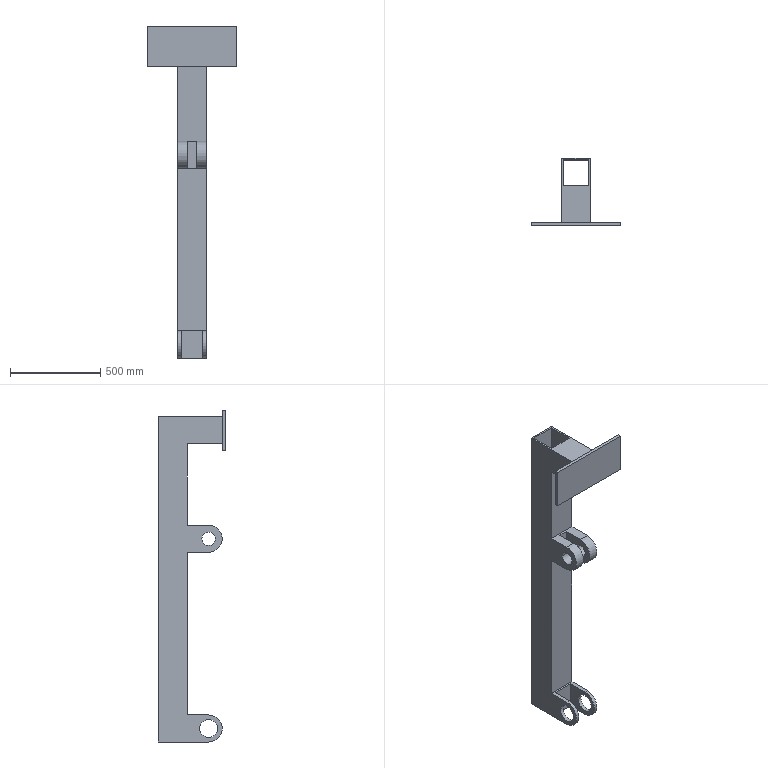Part | SolidWorks | features BaseBody 1 | 1 solid | 39 faces | box 495 x 375.221 x 1838 mm | volume 21198694 mm3 | plane 27 | cylinder 12 | commonest cylinder face diameters 75 x4 100 x4 150 x4
STEP:
#1=CARTESIAN_POINT('',(25.,-237.5,1125.));
#2=VERTEX_POINT('',#1);
#3=CARTESIAN_POINT('',(25.,-162.5,1125.));
#4=VERTEX_POINT('',#3);
#5=CARTESIAN_POINT('',(25.,-200.,1125.));
#6=DIRECTION('',(1.,0.,0.));
#7=DIRECTION('',(0.,1.,0.));
#8=AXIS2_PLACEMENT_3D('',#5,#6,#7);
#9=CIRCLE('',#8,37.5);
#10=EDGE_CURVE('',#2,#4,#9,.T.);
#11=ORIENTED_EDGE('',*,*,#10,.F.);
#12=CARTESIAN_POINT('',(80.,-237.5,1125.));
#13=VERTEX_POINT('',#12);
#14=CARTESIAN_POINT('',(-289.,-237.5,1125.));
#15=DIRECTION('',(1.,0.,0.));
#16=VECTOR('',#15,1000.);
#17=LINE('',#14,#16);
#18=EDGE_CURVE('',#2,#13,#17,.T.);
#19=ORIENTED_EDGE('',*,*,#18,.T.);
#20=CARTESIAN_POINT('',(80.,-162.5,1125.));
#21=VERTEX_POINT('',#20);
#22=CARTESIAN_POINT('',(80.,-200.,1125.));
#23=DIRECTION('',(1.,0.,0.));
#24=DIRECTION('',(0.,1.,0.));
#25=AXIS2_PLACEMENT_3D('',#22,#23,#24);
#26=CIRCLE('',#25,37.5);
#27=EDGE_CURVE('',#13,#21,#26,.T.);
#28=ORIENTED_EDGE('',*,*,#27,.T.);
#29=CARTESIAN_POINT('',(-289.,-162.5,1125.));
#30=DIRECTION('',(1.,0.,0.));
#31=VECTOR('',#30,1000.);
#32=LINE('',#29,#31);
#33=EDGE_CURVE('',#4,#21,#32,.T.);
#34=ORIENTED_EDGE('',*,*,#33,.F.);
#35=EDGE_LOOP('',(#11,#19,#28,#34));
#36=FACE_OUTER_BOUND('',#35,.T.);
#37=CARTESIAN_POINT('',(-289.,-200.,1125.));
#38=DIRECTION('',(1.,0.,0.));
#39=DIRECTION('',(0.,1.,0.));
#40=AXIS2_PLACEMENT_3D('',#37,#38,#39);
#41=CYLINDRICAL_SURFACE('',#40,37.5);
#42=ADVANCED_FACE('',(#36),#41,.F.);
#43=CARTESIAN_POINT('',(60.,-250.,75.));
#44=VERTEX_POINT('',#43);
#45=CARTESIAN_POINT('',(60.,-150.,75.));
#46=VERTEX_POINT('',#45);
#47=CARTESIAN_POINT('',(60.,-200.,75.));
#48=DIRECTION('',(1.,0.,0.));
#49=DIRECTION('',(0.,1.,0.));
#50=AXIS2_PLACEMENT_3D('',#47,#48,#49);
#51=CIRCLE('',#50,50.);
#52=EDGE_CURVE('',#44,#46,#51,.T.);
#53=ORIENTED_EDGE('',*,*,#52,.F.);
#54=CARTESIAN_POINT('',(80.,-250.,75.));
#55=VERTEX_POINT('',#54);
#56=CARTESIAN_POINT('',(-2456.,-250.,75.));
#57=DIRECTION('',(1.,0.,0.));
#58=VECTOR('',#57,1000.);
#59=LINE('',#56,#58);
#60=EDGE_CURVE('',#44,#55,#59,.T.);
#61=ORIENTED_EDGE('',*,*,#60,.T.);
#62=CARTESIAN_POINT('',(80.,-150.,75.));
#63=VERTEX_POINT('',#62);
#64=CARTESIAN_POINT('',(80.,-200.,75.));
#65=DIRECTION('',(1.,0.,0.));
#66=DIRECTION('',(0.,1.,0.));
#67=AXIS2_PLACEMENT_3D('',#64,#65,#66);
#68=CIRCLE('',#67,50.);
#69=EDGE_CURVE('',#55,#63,#68,.T.);
#70=ORIENTED_EDGE('',*,*,#69,.T.);
#71=CARTESIAN_POINT('',(-2456.,-150.,75.));
#72=DIRECTION('',(1.,0.,0.));
#73=VECTOR('',#72,1000.);
#74=LINE('',#71,#73);
#75=EDGE_CURVE('',#46,#63,#74,.T.);
#76=ORIENTED_EDGE('',*,*,#75,.F.);
#77=EDGE_LOOP('',(#53,#61,#70,#76));
#78=FACE_OUTER_BOUND('',#77,.T.);
#79=CARTESIAN_POINT('',(-2456.,-200.,75.));
#80=DIRECTION('',(1.,0.,0.));
#81=DIRECTION('',(0.,1.,0.));
#82=AXIS2_PLACEMENT_3D('',#79,#80,#81);
#83=CYLINDRICAL_SURFACE('',#82,50.);
#84=ADVANCED_FACE('',(#78),#83,.F.);
#85=CARTESIAN_POINT('',(-80.,-162.5,1125.));
#86=VERTEX_POINT('',#85);
#87=CARTESIAN_POINT('',(-80.,-237.5,1125.));
#88=VERTEX_POINT('',#87);
#89=CARTESIAN_POINT('',(-80.,-200.,1125.));
#90=DIRECTION('',(-1.,0.,0.));
#91=DIRECTION('',(0.,1.,0.));
#92=AXIS2_PLACEMENT_3D('',#89,#90,#91);
#93=CIRCLE('',#92,37.5);
#94=EDGE_CURVE('',#86,#88,#93,.T.);
#95=ORIENTED_EDGE('',*,*,#94,.T.);
#96=CARTESIAN_POINT('',(-25.,-237.5,1125.));
#97=VERTEX_POINT('',#96);
#98=CARTESIAN_POINT('',(-289.,-237.5,1125.));
#99=DIRECTION('',(1.,0.,0.));
#100=VECTOR('',#99,1000.);
#101=LINE('',#98,#100);
#102=EDGE_CURVE('',#88,#97,#101,.T.);
#103=ORIENTED_EDGE('',*,*,#102,.T.);
#104=CARTESIAN_POINT('',(-25.,-162.5,1125.));
#105=VERTEX_POINT('',#104);
#106=CARTESIAN_POINT('',(-25.,-200.,1125.));
#107=DIRECTION('',(-1.,0.,0.));
#108=DIRECTION('',(0.,1.,0.));
#109=AXIS2_PLACEMENT_3D('',#106,#107,#108);
#110=CIRCLE('',#109,37.5);
#111=EDGE_CURVE('',#105,#97,#110,.T.);
#112=ORIENTED_EDGE('',*,*,#111,.F.);
#113=CARTESIAN_POINT('',(-289.,-162.5,1125.));
#114=DIRECTION('',(1.,0.,0.));
#115=VECTOR('',#114,1000.);
#116=LINE('',#113,#115);
#117=EDGE_CURVE('',#86,#105,#116,.T.);
#118=ORIENTED_EDGE('',*,*,#117,.F.);
#119=EDGE_LOOP('',(#95,#103,#112,#118));
#120=FACE_OUTER_BOUND('',#119,.T.);
#121=CARTESIAN_POINT('',(-289.,-200.,1125.));
#122=DIRECTION('',(1.,0.,0.));
#123=DIRECTION('',(0.,1.,0.));
#124=AXIS2_PLACEMENT_3D('',#121,#122,#123);
#125=CYLINDRICAL_SURFACE('',#124,37.5);
#126=ADVANCED_FACE('',(#120),#125,.F.);
#127=CARTESIAN_POINT('',(-80.,-150.,75.));
#128=VERTEX_POINT('',#127);
#129=CARTESIAN_POINT('',(-80.,-250.,75.));
#130=VERTEX_POINT('',#129);
#131=CARTESIAN_POINT('',(-80.,-200.,75.));
#132=DIRECTION('',(-1.,0.,0.));
#133=DIRECTION('',(0.,1.,0.));
#134=AXIS2_PLACEMENT_3D('',#131,#132,#133);
#135=CIRCLE('',#134,50.);
#136=EDGE_CURVE('',#128,#130,#135,.T.);
#137=ORIENTED_EDGE('',*,*,#136,.T.);
#138=CARTESIAN_POINT('',(-60.,-250.,75.));
#139=VERTEX_POINT('',#138);
#140=CARTESIAN_POINT('',(-2456.,-250.,75.));
#141=DIRECTION('',(1.,0.,0.));
#142=VECTOR('',#141,1000.);
#143=LINE('',#140,#142);
#144=EDGE_CURVE('',#130,#139,#143,.T.);
#145=ORIENTED_EDGE('',*,*,#144,.T.);
#146=CARTESIAN_POINT('',(-60.,-150.,75.));
#147=VERTEX_POINT('',#146);
#148=CARTESIAN_POINT('',(-60.,-200.,75.));
#149=DIRECTION('',(1.,0.,0.));
#150=DIRECTION('',(0.,1.,0.));
#151=AXIS2_PLACEMENT_3D('',#148,#149,#150);
#152=CIRCLE('',#151,50.);
#153=EDGE_CURVE('',#139,#147,#152,.T.);
#154=ORIENTED_EDGE('',*,*,#153,.T.);
#155=CARTESIAN_POINT('',(-2456.,-150.,75.));
#156=DIRECTION('',(1.,0.,0.));
#157=VECTOR('',#156,1000.);
#158=LINE('',#155,#157);
#159=EDGE_CURVE('',#128,#147,#158,.T.);
#160=ORIENTED_EDGE('',*,*,#159,.F.);
#161=EDGE_LOOP('',(#137,#145,#154,#160));
#162=FACE_OUTER_BOUND('',#161,.T.);
#163=CARTESIAN_POINT('',(-2456.,-200.,75.));
#164=DIRECTION('',(1.,0.,0.));
#165=DIRECTION('',(0.,1.,0.));
#166=AXIS2_PLACEMENT_3D('',#163,#164,#165);
#167=CYLINDRICAL_SURFACE('',#166,50.);
#168=ADVANCED_FACE('',(#162),#167,.F.);
#169=CARTESIAN_POINT('',(80.,-200.,1125.));
#170=DIRECTION('',(1.,0.,0.));
#171=DIRECTION('',(0.,1.,0.));
#172=AXIS2_PLACEMENT_3D('',#169,#170,#171);
#173=CIRCLE('',#172,37.5);
#174=EDGE_CURVE('',#21,#13,#173,.T.);
#175=ORIENTED_EDGE('',*,*,#174,.F.);
#176=ORIENTED_EDGE('',*,*,#27,.F.);
#177=EDGE_LOOP('',(#175,#176));
#178=FACE_BOUND('',#177,.T.);
#179=CARTESIAN_POINT('',(80.,-200.,75.));
#180=DIRECTION('',(1.,0.,0.));
#181=DIRECTION('',(0.,1.,0.));
#182=AXIS2_PLACEMENT_3D('',#179,#180,#181);
#183=CIRCLE('',#182,50.);
#184=EDGE_CURVE('',#63,#55,#183,.T.);
#185=ORIENTED_EDGE('',*,*,#184,.F.);
#186=ORIENTED_EDGE('',*,*,#69,.F.);
#187=EDGE_LOOP('',(#185,#186));
#188=FACE_BOUND('',#187,.T.);
#189=CARTESIAN_POINT('',(80.,-80.,1200.));
#190=VERTEX_POINT('',#189);
#191=CARTESIAN_POINT('',(80.,-80.,1650.));
#192=VERTEX_POINT('',#191);
#193=CARTESIAN_POINT('',(80.,-80.,1800.));
#194=DIRECTION('',(0.,0.,1.));
#195=VECTOR('',#194,1000.);
#196=LINE('',#193,#195);
#197=EDGE_CURVE('',#190,#192,#196,.T.);
#198=ORIENTED_EDGE('',*,*,#197,.F.);
#199=CARTESIAN_POINT('',(80.,-200.,1200.));
#200=VERTEX_POINT('',#199);
#201=CARTESIAN_POINT('',(80.,-80.,1200.));
#202=DIRECTION('',(0.,1.,0.));
#203=VECTOR('',#202,1000.);
#204=LINE('',#201,#203);
#205=EDGE_CURVE('',#200,#190,#204,.T.);
#206=ORIENTED_EDGE('',*,*,#205,.F.);
#207=CARTESIAN_POINT('',(80.,-200.,1050.));
#208=VERTEX_POINT('',#207);
#209=CARTESIAN_POINT('',(80.,-200.,1125.));
#210=DIRECTION('',(-1.,0.,0.));
#211=DIRECTION('',(0.,1.,0.));
#212=AXIS2_PLACEMENT_3D('',#209,#210,#211);
#213=CIRCLE('',#212,75.);
#214=EDGE_CURVE('',#208,#200,#213,.T.);
#215=ORIENTED_EDGE('',*,*,#214,.F.);
#216=CARTESIAN_POINT('',(80.,-80.,1050.));
#217=VERTEX_POINT('',#216);
#218=CARTESIAN_POINT('',(80.,-80.,1050.));
#219=DIRECTION('',(0.,-1.,0.));
#220=VECTOR('',#219,1000.);
#221=LINE('',#218,#220);
#222=EDGE_CURVE('',#217,#208,#221,.T.);
#223=ORIENTED_EDGE('',*,*,#222,.F.);
#224=CARTESIAN_POINT('',(80.,-80.,150.));
#225=VERTEX_POINT('',#224);
#226=CARTESIAN_POINT('',(80.,-80.,1800.));
#227=DIRECTION('',(0.,0.,1.));
#228=VECTOR('',#227,1000.);
#229=LINE('',#226,#228);
#230=EDGE_CURVE('',#225,#217,#229,.T.);
#231=ORIENTED_EDGE('',*,*,#230,.F.);
#232=CARTESIAN_POINT('',(80.,-200.,150.));
#233=VERTEX_POINT('',#232);
#234=CARTESIAN_POINT('',(80.,-80.,150.));
#235=DIRECTION('',(0.,1.,0.));
#236=VECTOR('',#235,1000.);
#237=LINE('',#234,#236);
#238=EDGE_CURVE('',#233,#225,#237,.T.);
#239=ORIENTED_EDGE('',*,*,#238,.F.);
#240=CARTESIAN_POINT('',(80.,-200.,0.));
#241=VERTEX_POINT('',#240);
#242=CARTESIAN_POINT('',(80.,-200.,75.));
#243=DIRECTION('',(-1.,0.,0.));
#244=DIRECTION('',(0.,1.,0.));
#245=AXIS2_PLACEMENT_3D('',#242,#243,#244);
#246=CIRCLE('',#245,75.);
#247=EDGE_CURVE('',#241,#233,#246,.T.);
#248=ORIENTED_EDGE('',*,*,#247,.F.);
#249=CARTESIAN_POINT('',(80.,80.,0.));
#250=VERTEX_POINT('',#249);
#251=CARTESIAN_POINT('',(80.,-80.,0.));
#252=DIRECTION('',(0.,-1.,0.));
#253=VECTOR('',#252,1000.);
#254=LINE('',#251,#253);
#255=EDGE_CURVE('',#250,#241,#254,.T.);
#256=ORIENTED_EDGE('',*,*,#255,.F.);
#257=CARTESIAN_POINT('',(80.,80.,1800.));
#258=VERTEX_POINT('',#257);
#259=CARTESIAN_POINT('',(80.,80.,1800.));
#260=DIRECTION('',(0.,0.,-1.));
#261=VECTOR('',#260,1000.);
#262=LINE('',#259,#261);
#263=EDGE_CURVE('',#258,#250,#262,.T.);
#264=ORIENTED_EDGE('',*,*,#263,.F.);
#265=CARTESIAN_POINT('',(80.,-275.221,1800.));
#266=VERTEX_POINT('',#265);
#267=CARTESIAN_POINT('',(80.,-80.,1800.));
#268=DIRECTION('',(0.,1.,0.));
#269=VECTOR('',#268,1000.);
#270=LINE('',#267,#269);
#271=EDGE_CURVE('',#266,#258,#270,.T.);
#272=ORIENTED_EDGE('',*,*,#271,.F.);
#273=CARTESIAN_POINT('',(80.,-275.221,1650.));
#274=VERTEX_POINT('',#273);
#275=CARTESIAN_POINT('',(80.,-275.221,1800.));
#276=DIRECTION('',(0.,0.,1.));
#277=VECTOR('',#276,1000.);
#278=LINE('',#275,#277);
#279=EDGE_CURVE('',#274,#266,#278,.T.);
#280=ORIENTED_EDGE('',*,*,#279,.F.);
#281=CARTESIAN_POINT('',(80.,-80.,1650.));
#282=DIRECTION('',(0.,-1.,0.));
#283=VECTOR('',#282,1000.);
#284=LINE('',#281,#283);
#285=EDGE_CURVE('',#192,#274,#284,.T.);
#286=ORIENTED_EDGE('',*,*,#285,.F.);
#287=EDGE_LOOP('',(#198,#206,#215,#223,#231,#239,#248,#256,#264,#272,#280,#286));
#288=FACE_OUTER_BOUND('',#287,.T.);
#289=CARTESIAN_POINT('',(80.,-80.,1800.));
#290=DIRECTION('',(-1.,0.,0.));
#291=DIRECTION('',(0.,-1.,0.));
#292=AXIS2_PLACEMENT_3D('',#289,#290,#291);
#293=PLANE('',#292);
#294=ADVANCED_FACE('',(#178,#188,#288),#293,.F.);
#295=ORIENTED_EDGE('',*,*,#18,.F.);
#296=CARTESIAN_POINT('',(25.,-200.,1125.));
#297=DIRECTION('',(1.,0.,0.));
#298=DIRECTION('',(0.,1.,0.));
#299=AXIS2_PLACEMENT_3D('',#296,#297,#298);
#300=CIRCLE('',#299,37.5);
#301=EDGE_CURVE('',#4,#2,#300,.T.);
#302=ORIENTED_EDGE('',*,*,#301,.F.);
#303=ORIENTED_EDGE('',*,*,#33,.T.);
#304=ORIENTED_EDGE('',*,*,#174,.T.);
#305=EDGE_LOOP('',(#295,#302,#303,#304));
#306=FACE_OUTER_BOUND('',#305,.T.);
#307=CARTESIAN_POINT('',(-289.,-200.,1125.));
#308=DIRECTION('',(1.,0.,0.));
#309=DIRECTION('',(0.,1.,0.));
#310=AXIS2_PLACEMENT_3D('',#307,#308,#309);
#311=CYLINDRICAL_SURFACE('',#310,37.5);
#312=ADVANCED_FACE('',(#306),#311,.F.);
#313=ORIENTED_EDGE('',*,*,#60,.F.);
#314=CARTESIAN_POINT('',(60.,-200.,75.));
#315=DIRECTION('',(1.,0.,0.));
#316=DIRECTION('',(0.,1.,0.));
#317=AXIS2_PLACEMENT_3D('',#314,#315,#316);
#318=CIRCLE('',#317,50.);
#319=EDGE_CURVE('',#46,#44,#318,.T.);
#320=ORIENTED_EDGE('',*,*,#319,.F.);
#321=ORIENTED_EDGE('',*,*,#75,.T.);
#322=ORIENTED_EDGE('',*,*,#184,.T.);
#323=EDGE_LOOP('',(#313,#320,#321,#322));
#324=FACE_OUTER_BOUND('',#323,.T.);
#325=CARTESIAN_POINT('',(-2456.,-200.,75.));
#326=DIRECTION('',(1.,0.,0.));
#327=DIRECTION('',(0.,1.,0.));
#328=AXIS2_PLACEMENT_3D('',#325,#326,#327);
#329=CYLINDRICAL_SURFACE('',#328,50.);
#330=ADVANCED_FACE('',(#324),#329,.F.);
#331=ORIENTED_EDGE('',*,*,#285,.T.);
#332=CARTESIAN_POINT('',(-80.,-275.221,1650.));
#333=VERTEX_POINT('',#332);
#334=CARTESIAN_POINT('',(-80.,-275.221,1650.));
#335=DIRECTION('',(-1.,0.,0.));
#336=VECTOR('',#335,1000.);
#337=LINE('',#334,#336);
#338=EDGE_CURVE('',#274,#333,#337,.T.);
#339=ORIENTED_EDGE('',*,*,#338,.T.);
#340=CARTESIAN_POINT('',(-80.,-80.,1650.));
#341=VERTEX_POINT('',#340);
#342=CARTESIAN_POINT('',(-80.,-200.,1650.));
#343=DIRECTION('',(0.,1.,0.));
#344=VECTOR('',#343,1000.);
#345=LINE('',#342,#344);
#346=EDGE_CURVE('',#333,#341,#345,.T.);
#347=ORIENTED_EDGE('',*,*,#346,.T.);
#348=CARTESIAN_POINT('',(-80.,-80.,1650.));
#349=DIRECTION('',(1.,0.,0.));
#350=VECTOR('',#349,1000.);
#351=LINE('',#348,#350);
#352=EDGE_CURVE('',#341,#192,#351,.T.);
#353=ORIENTED_EDGE('',*,*,#352,.T.);
#354=EDGE_LOOP('',(#331,#339,#347,#353));
#355=FACE_OUTER_BOUND('',#354,.T.);
#356=CARTESIAN_POINT('',(-80.,-200.,1650.));
#357=DIRECTION('',(0.,0.,-1.));
#358=DIRECTION('',(0.,1.,0.));
#359=AXIS2_PLACEMENT_3D('',#356,#357,#358);
#360=PLANE('',#359);
#361=ADVANCED_FACE('',(#355),#360,.T.);
#362=ORIENTED_EDGE('',*,*,#352,.F.);
#363=CARTESIAN_POINT('',(-80.,-80.,1200.));
#364=VERTEX_POINT('',#363);
#365=CARTESIAN_POINT('',(-80.,-80.,1800.));
#366=DIRECTION('',(0.,0.,1.));
#367=VECTOR('',#366,1000.);
#368=LINE('',#365,#367);
#369=EDGE_CURVE('',#364,#341,#368,.T.);
#370=ORIENTED_EDGE('',*,*,#369,.F.);
#371=CARTESIAN_POINT('',(80.,-80.,1200.));
#372=DIRECTION('',(-1.,0.,0.));
#373=VECTOR('',#372,1000.);
#374=LINE('',#371,#373);
#375=EDGE_CURVE('',#190,#364,#374,.T.);
#376=ORIENTED_EDGE('',*,*,#375,.F.);
#377=ORIENTED_EDGE('',*,*,#197,.T.);
#378=EDGE_LOOP('',(#362,#370,#376,#377));
#379=FACE_OUTER_BOUND('',#378,.T.);
#380=CARTESIAN_POINT('',(80.,-80.,1800.));
#381=DIRECTION('',(0.,1.,0.));
#382=DIRECTION('',(-1.,0.,0.));
#383=AXIS2_PLACEMENT_3D('',#380,#381,#382);
#384=PLANE('',#383);
#385=ADVANCED_FACE('',(#379),#384,.F.);
#386=CARTESIAN_POINT('',(-80.,-200.,1200.));
#387=VERTEX_POINT('',#386);
#388=CARTESIAN_POINT('',(-25.,-200.,1200.));
#389=VERTEX_POINT('',#388);
#390=CARTESIAN_POINT('',(-80.,-200.,1200.));
#391=DIRECTION('',(1.,0.,0.));
#392=VECTOR('',#391,1000.);
#393=LINE('',#390,#392);
#394=EDGE_CURVE('',#387,#389,#393,.T.);
#395=ORIENTED_EDGE('',*,*,#394,.T.);
#396=CARTESIAN_POINT('',(-25.,-90.221,1200.));
#397=VERTEX_POINT('',#396);
#398=CARTESIAN_POINT('',(-25.,-80.,1200.));
#399=DIRECTION('',(0.,1.,0.));
#400=VECTOR('',#399,1000.);
#401=LINE('',#398,#400);
#402=EDGE_CURVE('',#389,#397,#401,.T.);
#403=ORIENTED_EDGE('',*,*,#402,.T.);
#404=CARTESIAN_POINT('',(25.,-90.221,1200.));
#405=VERTEX_POINT('',#404);
#406=CARTESIAN_POINT('',(-80.,-90.221,1200.));
#407=DIRECTION('',(1.,0.,0.));
#408=VECTOR('',#407,1000.);
#409=LINE('',#406,#408);
#410=EDGE_CURVE('',#397,#405,#409,.T.);
#411=ORIENTED_EDGE('',*,*,#410,.T.);
#412=CARTESIAN_POINT('',(25.,-200.,1200.));
#413=VERTEX_POINT('',#412);
#414=CARTESIAN_POINT('',(25.,-80.,1200.));
#415=DIRECTION('',(0.,-1.,0.));
#416=VECTOR('',#415,1000.);
#417=LINE('',#414,#416);
#418=EDGE_CURVE('',#405,#413,#417,.T.);
#419=ORIENTED_EDGE('',*,*,#418,.T.);
#420=CARTESIAN_POINT('',(-80.,-200.,1200.));
#421=DIRECTION('',(1.,0.,0.));
#422=VECTOR('',#421,1000.);
#423=LINE('',#420,#422);
#424=EDGE_CURVE('',#413,#200,#423,.T.);
#425=ORIENTED_EDGE('',*,*,#424,.T.);
#426=ORIENTED_EDGE('',*,*,#205,.T.);
#427=ORIENTED_EDGE('',*,*,#375,.T.);
#428=CARTESIAN_POINT('',(-80.,-80.,1200.));
#429=DIRECTION('',(0.,-1.,0.));
#430=VECTOR('',#429,1000.);
#431=LINE('',#428,#430);
#432=EDGE_CURVE('',#364,#387,#431,.T.);
#433=ORIENTED_EDGE('',*,*,#432,.T.);
#434=EDGE_LOOP('',(#395,#403,#411,#419,#425,#426,#427,#433));
#435=FACE_OUTER_BOUND('',#434,.T.);
#436=CARTESIAN_POINT('',(-80.,-80.,1200.));
#437=DIRECTION('',(0.,0.,1.));
#438=DIRECTION('',(0.,-1.,0.));
#439=AXIS2_PLACEMENT_3D('',#436,#437,#438);
#440=PLANE('',#439);
#441=ADVANCED_FACE('',(#435),#440,.T.);
#442=CARTESIAN_POINT('',(25.,-200.,1050.));
#443=VERTEX_POINT('',#442);
#444=CARTESIAN_POINT('',(-80.,-200.,1050.));
#445=DIRECTION('',(1.,0.,0.));
#446=VECTOR('',#445,1000.);
#447=LINE('',#444,#446);
#448=EDGE_CURVE('',#443,#208,#447,.T.);
#449=ORIENTED_EDGE('',*,*,#448,.T.);
#450=ORIENTED_EDGE('',*,*,#214,.T.);
#451=ORIENTED_EDGE('',*,*,#424,.F.);
#452=CARTESIAN_POINT('',(25.,-200.,1125.));
#453=DIRECTION('',(1.,0.,0.));
#454=DIRECTION('',(0.,1.,0.));
#455=AXIS2_PLACEMENT_3D('',#452,#453,#454);
#456=CIRCLE('',#455,75.);
#457=EDGE_CURVE('',#413,#443,#456,.T.);
#458=ORIENTED_EDGE('',*,*,#457,.T.);
#459=EDGE_LOOP('',(#449,#450,#451,#458));
#460=FACE_OUTER_BOUND('',#459,.T.);
#461=CARTESIAN_POINT('',(-80.,-200.,1125.));
#462=DIRECTION('',(1.,0.,0.));
#463=DIRECTION('',(0.,1.,0.));
#464=AXIS2_PLACEMENT_3D('',#461,#462,#463);
#465=CYLINDRICAL_SURFACE('',#464,75.);
#466=ADVANCED_FACE('',(#460),#465,.T.);
#467=CARTESIAN_POINT('',(-80.,-80.,1050.));
#468=VERTEX_POINT('',#467);
#469=CARTESIAN_POINT('',(-80.,-80.,1050.));
#470=DIRECTION('',(1.,0.,0.));
#471=VECTOR('',#470,1000.);
#472=LINE('',#469,#471);
#473=EDGE_CURVE('',#468,#217,#472,.T.);
#474=ORIENTED_EDGE('',*,*,#473,.T.);
#475=ORIENTED_EDGE('',*,*,#222,.T.);
#476=ORIENTED_EDGE('',*,*,#448,.F.);
#477=CARTESIAN_POINT('',(25.,-90.221,1050.));
#478=VERTEX_POINT('',#477);
#479=CARTESIAN_POINT('',(25.,-200.,1050.));
#480=DIRECTION('',(0.,1.,0.));
#481=VECTOR('',#480,1000.);
#482=LINE('',#479,#481);
#483=EDGE_CURVE('',#443,#478,#482,.T.);
#484=ORIENTED_EDGE('',*,*,#483,.T.);
#485=CARTESIAN_POINT('',(-25.,-90.221,1050.));
#486=VERTEX_POINT('',#485);
#487=CARTESIAN_POINT('',(-80.,-90.221,1050.));
#488=DIRECTION('',(-1.,0.,0.));
#489=VECTOR('',#488,1000.);
#490=LINE('',#487,#489);
#491=EDGE_CURVE('',#478,#486,#490,.T.);
#492=ORIENTED_EDGE('',*,*,#491,.T.);
#493=CARTESIAN_POINT('',(-25.,-200.,1050.));
#494=VERTEX_POINT('',#493);
#495=CARTESIAN_POINT('',(-25.,-200.,1050.));
#496=DIRECTION('',(0.,-1.,0.));
#497=VECTOR('',#496,1000.);
#498=LINE('',#495,#497);
#499=EDGE_CURVE('',#486,#494,#498,.T.);
#500=ORIENTED_EDGE('',*,*,#499,.T.);
#501=CARTESIAN_POINT('',(-80.,-200.,1050.));
#502=VERTEX_POINT('',#501);
#503=CARTESIAN_POINT('',(-80.,-200.,1050.));
#504=DIRECTION('',(-1.,0.,0.));
#505=VECTOR('',#504,1000.);
#506=LINE('',#503,#505);
#507=EDGE_CURVE('',#494,#502,#506,.T.);
#508=ORIENTED_EDGE('',*,*,#507,.T.);
#509=CARTESIAN_POINT('',(-80.,-200.,1050.));
#510=DIRECTION('',(0.,1.,0.));
#511=VECTOR('',#510,1000.);
#512=LINE('',#509,#511);
#513=EDGE_CURVE('',#502,#468,#512,.T.);
#514=ORIENTED_EDGE('',*,*,#513,.T.);
#515=EDGE_LOOP('',(#474,#475,#476,#484,#492,#500,#508,#514));
#516=FACE_OUTER_BOUND('',#515,.T.);
#517=CARTESIAN_POINT('',(-80.,-200.,1050.));
#518=DIRECTION('',(0.,0.,-1.));
#519=DIRECTION('',(-1.,0.,0.));
#520=AXIS2_PLACEMENT_3D('',#517,#518,#519);
#521=PLANE('',#520);
#522=ADVANCED_FACE('',(#516),#521,.T.);
#523=ORIENTED_EDGE('',*,*,#473,.F.);
#524=CARTESIAN_POINT('',(-80.,-80.,150.));
#525=VERTEX_POINT('',#524);
#526=CARTESIAN_POINT('',(-80.,-80.,1800.));
#527=DIRECTION('',(0.,0.,1.));
#528=VECTOR('',#527,1000.);
#529=LINE('',#526,#528);
#530=EDGE_CURVE('',#525,#468,#529,.T.);
#531=ORIENTED_EDGE('',*,*,#530,.F.);
#532=CARTESIAN_POINT('',(80.,-80.,150.));
#533=DIRECTION('',(-1.,0.,0.));
#534=VECTOR('',#533,1000.);
#535=LINE('',#532,#534);
#536=EDGE_CURVE('',#225,#525,#535,.T.);
#537=ORIENTED_EDGE('',*,*,#536,.F.);
#538=ORIENTED_EDGE('',*,*,#230,.T.);
#539=EDGE_LOOP('',(#523,#531,#537,#538));
#540=FACE_OUTER_BOUND('',#539,.T.);
#541=CARTESIAN_POINT('',(80.,-80.,1800.));
#542=DIRECTION('',(0.,1.,0.));
#543=DIRECTION('',(-1.,0.,0.));
#544=AXIS2_PLACEMENT_3D('',#541,#542,#543);
#545=PLANE('',#544);
#546=ADVANCED_FACE('',(#540),#545,.F.);
#547=CARTESIAN_POINT('',(-60.,-200.,150.));
#548=VERTEX_POINT('',#547);
#549=CARTESIAN_POINT('',(-60.,-90.221,150.));
#550=VERTEX_POINT('',#549);
#551=CARTESIAN_POINT('',(-60.,-200.,150.));
#552=DIRECTION('',(0.,1.,0.));
#553=VECTOR('',#552,1000.);
#554=LINE('',#551,#553);
#555=EDGE_CURVE('',#548,#550,#554,.T.);
#556=ORIENTED_EDGE('',*,*,#555,.T.);
#557=CARTESIAN_POINT('',(60.,-90.221,150.));
#558=VERTEX_POINT('',#557);
#559=CARTESIAN_POINT('',(-80.,-90.221,150.));
#560=DIRECTION('',(1.,0.,0.));
#561=VECTOR('',#560,1000.);
#562=LINE('',#559,#561);
#563=EDGE_CURVE('',#550,#558,#562,.T.);
#564=ORIENTED_EDGE('',*,*,#563,.T.);
#565=CARTESIAN_POINT('',(60.,-200.,150.));
#566=VERTEX_POINT('',#565);
#567=CARTESIAN_POINT('',(60.,-200.,150.));
#568=DIRECTION('',(0.,-1.,0.));
#569=VECTOR('',#568,1000.);
#570=LINE('',#567,#569);
#571=EDGE_CURVE('',#558,#566,#570,.T.);
#572=ORIENTED_EDGE('',*,*,#571,.T.);
#573=CARTESIAN_POINT('',(-80.,-200.,150.));
#574=DIRECTION('',(1.,0.,0.));
#575=VECTOR('',#574,1000.);
#576=LINE('',#573,#575);
#577=EDGE_CURVE('',#566,#233,#576,.T.);
#578=ORIENTED_EDGE('',*,*,#577,.T.);
#579=ORIENTED_EDGE('',*,*,#238,.T.);
#580=ORIENTED_EDGE('',*,*,#536,.T.);
#581=CARTESIAN_POINT('',(-80.,-200.,150.));
#582=VERTEX_POINT('',#581);
#583=CARTESIAN_POINT('',(-80.,-200.,150.));
#584=DIRECTION('',(0.,-1.,0.));
#585=VECTOR('',#584,1000.);
#586=LINE('',#583,#585);
#587=EDGE_CURVE('',#525,#582,#586,.T.);
#588=ORIENTED_EDGE('',*,*,#587,.T.);
#589=CARTESIAN_POINT('',(-80.,-200.,150.));
#590=DIRECTION('',(1.,0.,0.));
#591=VECTOR('',#590,1000.);
#592=LINE('',#589,#591);
#593=EDGE_CURVE('',#582,#548,#592,.T.);
#594=ORIENTED_EDGE('',*,*,#593,.T.);
#595=EDGE_LOOP('',(#556,#564,#572,#578,#579,#580,#588,#594));
#596=FACE_OUTER_BOUND('',#595,.T.);
#597=CARTESIAN_POINT('',(-80.,-200.,150.));
#598=DIRECTION('',(0.,0.,1.));
#599=DIRECTION('',(0.,-1.,0.));
#600=AXIS2_PLACEMENT_3D('',#597,#598,#599);
#601=PLANE('',#600);
#602=ADVANCED_FACE('',(#596),#601,.T.);
#603=ORIENTED_EDGE('',*,*,#247,.T.);
#604=ORIENTED_EDGE('',*,*,#577,.F.);
#605=CARTESIAN_POINT('',(60.,-200.,0.));
#606=VERTEX_POINT('',#605);
#607=CARTESIAN_POINT('',(60.,-200.,75.));
#608=DIRECTION('',(1.,0.,0.));
#609=DIRECTION('',(0.,1.,0.));
#610=AXIS2_PLACEMENT_3D('',#607,#608,#609);
#611=CIRCLE('',#610,75.);
#612=EDGE_CURVE('',#566,#606,#611,.T.);
#613=ORIENTED_EDGE('',*,*,#612,.T.);
#614=CARTESIAN_POINT('',(-80.,-200.,0.));
#615=DIRECTION('',(1.,0.,0.));
#616=VECTOR('',#615,1000.);
#617=LINE('',#614,#616);
#618=EDGE_CURVE('',#606,#241,#617,.T.);
#619=ORIENTED_EDGE('',*,*,#618,.T.);
#620=EDGE_LOOP('',(#603,#604,#613,#619));
#621=FACE_OUTER_BOUND('',#620,.T.);
#622=CARTESIAN_POINT('',(-80.,-200.,75.));
#623=DIRECTION('',(1.,0.,0.));
#624=DIRECTION('',(0.,1.,0.));
#625=AXIS2_PLACEMENT_3D('',#622,#623,#624);
#626=CYLINDRICAL_SURFACE('',#625,75.);
#627=ADVANCED_FACE('',(#621),#626,.T.);
#628=CARTESIAN_POINT('',(-70.,70.,0.));
#629=VERTEX_POINT('',#628);
#630=CARTESIAN_POINT('',(70.,70.,0.));
#631=VERTEX_POINT('',#630);
#632=CARTESIAN_POINT('',(0.,70.,0.));
#633=DIRECTION('',(1.,0.,0.));
#634=VECTOR('',#633,1000.);
#635=LINE('',#632,#634);
#636=EDGE_CURVE('',#629,#631,#635,.T.);
#637=ORIENTED_EDGE('',*,*,#636,.F.);
#638=CARTESIAN_POINT('',(-70.,-70.,0.));
#639=VERTEX_POINT('',#638);
#640=CARTESIAN_POINT('',(-70.,0.,0.));
#641=DIRECTION('',(0.,1.,0.));
#642=VECTOR('',#641,1000.);
#643=LINE('',#640,#642);
#644=EDGE_CURVE('',#639,#629,#643,.T.);
#645=ORIENTED_EDGE('',*,*,#644,.F.);
#646=CARTESIAN_POINT('',(70.,-70.,0.));
#647=VERTEX_POINT('',#646);
#648=CARTESIAN_POINT('',(0.,-70.,0.));
#649=DIRECTION('',(-1.,0.,0.));
#650=VECTOR('',#649,1000.);
#651=LINE('',#648,#650);
#652=EDGE_CURVE('',#647,#639,#651,.T.);
#653=ORIENTED_EDGE('',*,*,#652,.F.);
#654=CARTESIAN_POINT('',(70.,0.,0.));
#655=DIRECTION('',(0.,-1.,0.));
#656=VECTOR('',#655,1000.);
#657=LINE('',#654,#656);
#658=EDGE_CURVE('',#631,#647,#657,.T.);
#659=ORIENTED_EDGE('',*,*,#658,.F.);
#660=EDGE_LOOP('',(#637,#645,#653,#659));
#661=FACE_BOUND('',#660,.T.);
#662=CARTESIAN_POINT('',(60.,-90.221,0.));
#663=VERTEX_POINT('',#662);
#664=CARTESIAN_POINT('',(60.,0.,0.));
#665=DIRECTION('',(0.,-1.,0.));
#666=VECTOR('',#665,1000.);
#667=LINE('',#664,#666);
#668=EDGE_CURVE('',#663,#606,#667,.T.);
#669=ORIENTED_EDGE('',*,*,#668,.F.);
#670=CARTESIAN_POINT('',(-60.,-90.221,0.));
#671=VERTEX_POINT('',#670);
#672=CARTESIAN_POINT('',(0.,-90.221,0.));
#673=DIRECTION('',(1.,0.,0.));
#674=VECTOR('',#673,1000.);
#675=LINE('',#672,#674);
#676=EDGE_CURVE('',#671,#663,#675,.T.);
#677=ORIENTED_EDGE('',*,*,#676,.F.);
#678=CARTESIAN_POINT('',(-60.,-200.,0.));
#679=VERTEX_POINT('',#678);
#680=CARTESIAN_POINT('',(-60.,0.,0.));
#681=DIRECTION('',(0.,1.,0.));
#682=VECTOR('',#681,1000.);
#683=LINE('',#680,#682);
#684=EDGE_CURVE('',#679,#671,#683,.T.);
#685=ORIENTED_EDGE('',*,*,#684,.F.);
#686=CARTESIAN_POINT('',(-80.,-200.,0.));
#687=VERTEX_POINT('',#686);
#688=CARTESIAN_POINT('',(0.,-200.,0.));
#689=DIRECTION('',(1.,0.,0.));
#690=VECTOR('',#689,1000.);
#691=LINE('',#688,#690);
#692=EDGE_CURVE('',#687,#679,#691,.T.);
#693=ORIENTED_EDGE('',*,*,#692,.F.);
#694=CARTESIAN_POINT('',(-80.,80.,0.));
#695=VERTEX_POINT('',#694);
#696=CARTESIAN_POINT('',(-80.,0.,0.));
#697=DIRECTION('',(0.,-1.,0.));
#698=VECTOR('',#697,1000.);
#699=LINE('',#696,#698);
#700=EDGE_CURVE('',#695,#687,#699,.T.);
#701=ORIENTED_EDGE('',*,*,#700,.F.);
#702=CARTESIAN_POINT('',(0.,80.,0.));
#703=DIRECTION('',(-1.,0.,0.));
#704=VECTOR('',#703,1000.);
#705=LINE('',#702,#704);
#706=EDGE_CURVE('',#250,#695,#705,.T.);
#707=ORIENTED_EDGE('',*,*,#706,.F.);
#708=ORIENTED_EDGE('',*,*,#255,.T.);
#709=ORIENTED_EDGE('',*,*,#618,.F.);
#710=EDGE_LOOP('',(#669,#677,#685,#693,#701,#707,#708,#709));
#711=FACE_OUTER_BOUND('',#710,.T.);
#712=CARTESIAN_POINT('',(0.,0.,0.));
#713=DIRECTION('',(0.,0.,1.));
#714=DIRECTION('',(1.,0.,0.));
#715=AXIS2_PLACEMENT_3D('',#712,#713,#714);
#716=PLANE('',#715);
#717=ADVANCED_FACE('',(#661,#711),#716,.F.);
#718=CARTESIAN_POINT('',(-80.,80.,1800.));
#719=VERTEX_POINT('',#718);
#720=CARTESIAN_POINT('',(-80.,80.,1800.));
#721=DIRECTION('',(0.,0.,-1.));
#722=VECTOR('',#721,1000.);
#723=LINE('',#720,#722);
#724=EDGE_CURVE('',#719,#695,#723,.T.);
#725=ORIENTED_EDGE('',*,*,#724,.F.);
#726=CARTESIAN_POINT('',(80.,80.,1800.));
#727=DIRECTION('',(-1.,0.,0.));
#728=VECTOR('',#727,1000.);
#729=LINE('',#726,#728);
#730=EDGE_CURVE('',#258,#719,#729,.T.);
#731=ORIENTED_EDGE('',*,*,#730,.F.);
#732=ORIENTED_EDGE('',*,*,#263,.T.);
#733=ORIENTED_EDGE('',*,*,#706,.T.);
#734=EDGE_LOOP('',(#725,#731,#732,#733));
#735=FACE_OUTER_BOUND('',#734,.T.);
#736=CARTESIAN_POINT('',(80.,80.,1800.));
#737=DIRECTION('',(0.,-1.,0.));
#738=DIRECTION('',(1.,0.,0.));
#739=AXIS2_PLACEMENT_3D('',#736,#737,#738);
#740=PLANE('',#739);
#741=ADVANCED_FACE('',(#735),#740,.F.);
#742=CARTESIAN_POINT('',(70.,-70.,1800.));
#743=VERTEX_POINT('',#742);
#744=CARTESIAN_POINT('',(-70.,-70.,1800.));
#745=VERTEX_POINT('',#744);
#746=CARTESIAN_POINT('',(0.,-70.,1800.));
#747=DIRECTION('',(-1.,0.,0.));
#748=VECTOR('',#747,1000.);
#749=LINE('',#746,#748);
#750=EDGE_CURVE('',#743,#745,#749,.T.);
#751=ORIENTED_EDGE('',*,*,#750,.T.);
#752=CARTESIAN_POINT('',(-70.,70.,1800.));
#753=VERTEX_POINT('',#752);
#754=CARTESIAN_POINT('',(-70.,0.,1800.));
#755=DIRECTION('',(0.,1.,0.));
#756=VECTOR('',#755,1000.);
#757=LINE('',#754,#756);
#758=EDGE_CURVE('',#745,#753,#757,.T.);
#759=ORIENTED_EDGE('',*,*,#758,.T.);
#760=CARTESIAN_POINT('',(70.,70.,1800.));
#761=VERTEX_POINT('',#760);
#762=CARTESIAN_POINT('',(0.,70.,1800.));
#763=DIRECTION('',(1.,0.,0.));
#764=VECTOR('',#763,1000.);
#765=LINE('',#762,#764);
#766=EDGE_CURVE('',#753,#761,#765,.T.);
#767=ORIENTED_EDGE('',*,*,#766,.T.);
#768=CARTESIAN_POINT('',(70.,0.,1800.));
#769=DIRECTION('',(0.,-1.,0.));
#770=VECTOR('',#769,1000.);
#771=LINE('',#768,#770);
#772=EDGE_CURVE('',#761,#743,#771,.T.);
#773=ORIENTED_EDGE('',*,*,#772,.T.);
#774=EDGE_LOOP('',(#751,#759,#767,#773));
#775=FACE_BOUND('',#774,.T.);
#776=CARTESIAN_POINT('',(-80.,-275.221,1800.));
#777=VERTEX_POINT('',#776);
#778=CARTESIAN_POINT('',(-80.,0.,1800.));
#779=DIRECTION('',(0.,-1.,0.));
#780=VECTOR('',#779,1000.);
#781=LINE('',#778,#780);
#782=EDGE_CURVE('',#719,#777,#781,.T.);
#783=ORIENTED_EDGE('',*,*,#782,.T.);
#784=CARTESIAN_POINT('',(0.,-275.221,1800.));
#785=DIRECTION('',(1.,0.,0.));
#786=VECTOR('',#785,1000.);
#787=LINE('',#784,#786);
#788=EDGE_CURVE('',#777,#266,#787,.T.);
#789=ORIENTED_EDGE('',*,*,#788,.T.);
#790=ORIENTED_EDGE('',*,*,#271,.T.);
#791=ORIENTED_EDGE('',*,*,#730,.T.);
#792=EDGE_LOOP('',(#783,#789,#790,#791));
#793=FACE_OUTER_BOUND('',#792,.T.);
#794=CARTESIAN_POINT('',(0.,0.,1800.));
#795=DIRECTION('',(0.,0.,1.));
#796=DIRECTION('',(1.,0.,0.));
#797=AXIS2_PLACEMENT_3D('',#794,#795,#796);
#798=PLANE('',#797);
#799=ADVANCED_FACE('',(#775,#793),#798,.T.);
#800=CARTESIAN_POINT('',(247.5,-275.221,1837.5));
#801=VERTEX_POINT('',#800);
#802=CARTESIAN_POINT('',(247.5,-275.221,1612.5));
#803=VERTEX_POINT('',#802);
#804=CARTESIAN_POINT('',(247.5,-275.221,0.));
#805=DIRECTION('',(0.,0.,-1.));
#806=VECTOR('',#805,1000.);
#807=LINE('',#804,#806);
#808=EDGE_CURVE('',#801,#803,#807,.T.);
#809=ORIENTED_EDGE('',*,*,#808,.T.);
#810=CARTESIAN_POINT('',(-247.5,-275.221,1612.5));
#811=VERTEX_POINT('',#810);
#812=CARTESIAN_POINT('',(0.,-275.221,1612.5));
#813=DIRECTION('',(-1.,0.,0.));
#814=VECTOR('',#813,1000.);
#815=LINE('',#812,#814);
#816=EDGE_CURVE('',#803,#811,#815,.T.);
#817=ORIENTED_EDGE('',*,*,#816,.T.);
#818=CARTESIAN_POINT('',(-247.5,-275.221,1837.5));
#819=VERTEX_POINT('',#818);
#820=CARTESIAN_POINT('',(-247.5,-275.221,0.));
#821=DIRECTION('',(0.,0.,1.));
#822=VECTOR('',#821,1000.);
#823=LINE('',#820,#822);
#824=EDGE_CURVE('',#811,#819,#823,.T.);
#825=ORIENTED_EDGE('',*,*,#824,.T.);
#826=CARTESIAN_POINT('',(0.,-275.221,1837.5));
#827=DIRECTION('',(1.,0.,0.));
#828=VECTOR('',#827,1000.);
#829=LINE('',#826,#828);
#830=EDGE_CURVE('',#819,#801,#829,.T.);
#831=ORIENTED_EDGE('',*,*,#830,.T.);
#832=EDGE_LOOP('',(#809,#817,#825,#831));
#833=FACE_OUTER_BOUND('',#832,.T.);
#834=ORIENTED_EDGE('',*,*,#338,.F.);
#835=ORIENTED_EDGE('',*,*,#279,.T.);
#836=ORIENTED_EDGE('',*,*,#788,.F.);
#837=CARTESIAN_POINT('',(-80.,-275.221,0.));
#838=DIRECTION('',(0.,0.,-1.));
#839=VECTOR('',#838,1000.);
#840=LINE('',#837,#839);
#841=EDGE_CURVE('',#777,#333,#840,.T.);
#842=ORIENTED_EDGE('',*,*,#841,.T.);
#843=EDGE_LOOP('',(#834,#835,#836,#842));
#844=FACE_BOUND('',#843,.T.);
#845=CARTESIAN_POINT('',(0.,-275.221,0.));
#846=DIRECTION('',(0.,1.,0.));
#847=DIRECTION('',(0.,0.,1.));
#848=AXIS2_PLACEMENT_3D('',#845,#846,#847);
#849=PLANE('',#848);
#850=ADVANCED_FACE('',(#833,#844),#849,.T.);
#851=ORIENTED_EDGE('',*,*,#301,.T.);
#852=ORIENTED_EDGE('',*,*,#10,.T.);
#853=EDGE_LOOP('',(#851,#852));
#854=FACE_BOUND('',#853,.T.);
#855=ORIENTED_EDGE('',*,*,#457,.F.);
#856=ORIENTED_EDGE('',*,*,#418,.F.);
#857=CARTESIAN_POINT('',(25.,-90.221,1125.));
#858=DIRECTION('',(0.,0.,-1.));
#859=VECTOR('',#858,1000.);
#860=LINE('',#857,#859);
#861=EDGE_CURVE('',#405,#478,#860,.T.);
#862=ORIENTED_EDGE('',*,*,#861,.T.);
#863=ORIENTED_EDGE('',*,*,#483,.F.);
#864=EDGE_LOOP('',(#855,#856,#862,#863));
#865=FACE_OUTER_BOUND('',#864,.T.);
#866=CARTESIAN_POINT('',(25.,-200.,1125.));
#867=DIRECTION('',(-1.,0.,0.));
#868=DIRECTION('',(0.,-1.,0.));
#869=AXIS2_PLACEMENT_3D('',#866,#867,#868);
#870=PLANE('',#869);
#871=ADVANCED_FACE('',(#854,#865),#870,.T.);
#872=ORIENTED_EDGE('',*,*,#571,.F.);
#873=CARTESIAN_POINT('',(60.,-90.221,2536.));
#874=DIRECTION('',(0.,0.,1.));
#875=VECTOR('',#874,1000.);
#876=LINE('',#873,#875);
#877=EDGE_CURVE('',#663,#558,#876,.T.);
#878=ORIENTED_EDGE('',*,*,#877,.F.);
#879=ORIENTED_EDGE('',*,*,#668,.T.);
#880=ORIENTED_EDGE('',*,*,#612,.F.);
#881=EDGE_LOOP('',(#872,#878,#879,#880));
#882=FACE_OUTER_BOUND('',#881,.T.);
#883=ORIENTED_EDGE('',*,*,#319,.T.);
#884=ORIENTED_EDGE('',*,*,#52,.T.);
#885=EDGE_LOOP('',(#883,#884));
#886=FACE_BOUND('',#885,.T.);
#887=CARTESIAN_POINT('',(60.,-275.,2536.));
#888=DIRECTION('',(1.,0.,0.));
#889=DIRECTION('',(0.,1.,0.));
#890=AXIS2_PLACEMENT_3D('',#887,#888,#889);
#891=PLANE('',#890);
#892=ADVANCED_FACE('',(#882,#886),#891,.F.);
#893=ORIENTED_EDGE('',*,*,#94,.F.);
#894=CARTESIAN_POINT('',(-80.,-200.,1125.));
#895=DIRECTION('',(-1.,0.,0.));
#896=DIRECTION('',(0.,1.,0.));
#897=AXIS2_PLACEMENT_3D('',#894,#895,#896);
#898=CIRCLE('',#897,37.5);
#899=EDGE_CURVE('',#88,#86,#898,.T.);
#900=ORIENTED_EDGE('',*,*,#899,.F.);
#901=EDGE_LOOP('',(#893,#900));
#902=FACE_BOUND('',#901,.T.);
#903=ORIENTED_EDGE('',*,*,#136,.F.);
#904=CARTESIAN_POINT('',(-80.,-200.,75.));
#905=DIRECTION('',(-1.,0.,0.));
#906=DIRECTION('',(0.,1.,0.));
#907=AXIS2_PLACEMENT_3D('',#904,#905,#906);
#908=CIRCLE('',#907,50.);
#909=EDGE_CURVE('',#130,#128,#908,.T.);
#910=ORIENTED_EDGE('',*,*,#909,.F.);
#911=EDGE_LOOP('',(#903,#910));
#912=FACE_BOUND('',#911,.T.);
#913=ORIENTED_EDGE('',*,*,#782,.F.);
#914=ORIENTED_EDGE('',*,*,#724,.T.);
#915=ORIENTED_EDGE('',*,*,#700,.T.);
#916=CARTESIAN_POINT('',(-80.,-200.,75.));
#917=DIRECTION('',(1.,0.,0.));
#918=DIRECTION('',(0.,1.,0.));
#919=AXIS2_PLACEMENT_3D('',#916,#917,#918);
#920=CIRCLE('',#919,75.);
#921=EDGE_CURVE('',#582,#687,#920,.T.);
#922=ORIENTED_EDGE('',*,*,#921,.F.);
#923=ORIENTED_EDGE('',*,*,#587,.F.);
#924=ORIENTED_EDGE('',*,*,#530,.T.);
#925=ORIENTED_EDGE('',*,*,#513,.F.);
#926=CARTESIAN_POINT('',(-80.,-200.,1125.));
#927=DIRECTION('',(1.,0.,0.));
#928=DIRECTION('',(0.,1.,0.));
#929=AXIS2_PLACEMENT_3D('',#926,#927,#928);
#930=CIRCLE('',#929,75.);
#931=EDGE_CURVE('',#387,#502,#930,.T.);
#932=ORIENTED_EDGE('',*,*,#931,.F.);
#933=ORIENTED_EDGE('',*,*,#432,.F.);
#934=ORIENTED_EDGE('',*,*,#369,.T.);
#935=ORIENTED_EDGE('',*,*,#346,.F.);
#936=ORIENTED_EDGE('',*,*,#841,.F.);
#937=EDGE_LOOP('',(#913,#914,#915,#922,#923,#924,#925,#932,#933,#934,#935,#936));
#938=FACE_OUTER_BOUND('',#937,.T.);
#939=CARTESIAN_POINT('',(-80.,-80.,1800.));
#940=DIRECTION('',(1.,0.,0.));
#941=DIRECTION('',(0.,1.,0.));
#942=AXIS2_PLACEMENT_3D('',#939,#940,#941);
#943=PLANE('',#942);
#944=ADVANCED_FACE('',(#902,#912,#938),#943,.F.);
#945=ORIENTED_EDGE('',*,*,#111,.T.);
#946=CARTESIAN_POINT('',(-25.,-200.,1125.));
#947=DIRECTION('',(-1.,0.,0.));
#948=DIRECTION('',(0.,1.,0.));
#949=AXIS2_PLACEMENT_3D('',#946,#947,#948);
#950=CIRCLE('',#949,37.5);
#951=EDGE_CURVE('',#97,#105,#950,.T.);
#952=ORIENTED_EDGE('',*,*,#951,.T.);
#953=EDGE_LOOP('',(#945,#952));
#954=FACE_BOUND('',#953,.T.);
#955=CARTESIAN_POINT('',(-25.,-90.221,1125.));
#956=DIRECTION('',(0.,0.,1.));
#957=VECTOR('',#956,1000.);
#958=LINE('',#955,#957);
#959=EDGE_CURVE('',#486,#397,#958,.T.);
#960=ORIENTED_EDGE('',*,*,#959,.T.);
#961=ORIENTED_EDGE('',*,*,#402,.F.);
#962=CARTESIAN_POINT('',(-25.,-200.,1125.));
#963=DIRECTION('',(1.,0.,0.));
#964=DIRECTION('',(0.,1.,0.));
#965=AXIS2_PLACEMENT_3D('',#962,#963,#964);
#966=CIRCLE('',#965,75.);
#967=EDGE_CURVE('',#389,#494,#966,.T.);
#968=ORIENTED_EDGE('',*,*,#967,.T.);
#969=ORIENTED_EDGE('',*,*,#499,.F.);
#970=EDGE_LOOP('',(#960,#961,#968,#969));
#971=FACE_OUTER_BOUND('',#970,.T.);
#972=CARTESIAN_POINT('',(-25.,-200.,1125.));
#973=DIRECTION('',(1.,0.,0.));
#974=DIRECTION('',(0.,1.,0.));
#975=AXIS2_PLACEMENT_3D('',#972,#973,#974);
#976=PLANE('',#975);
#977=ADVANCED_FACE('',(#954,#971),#976,.T.);
#978=ORIENTED_EDGE('',*,*,#394,.F.);
#979=ORIENTED_EDGE('',*,*,#931,.T.);
#980=ORIENTED_EDGE('',*,*,#507,.F.);
#981=ORIENTED_EDGE('',*,*,#967,.F.);
#982=EDGE_LOOP('',(#978,#979,#980,#981));
#983=FACE_OUTER_BOUND('',#982,.T.);
#984=CARTESIAN_POINT('',(-80.,-200.,1125.));
#985=DIRECTION('',(1.,0.,0.));
#986=DIRECTION('',(0.,1.,0.));
#987=AXIS2_PLACEMENT_3D('',#984,#985,#986);
#988=CYLINDRICAL_SURFACE('',#987,75.);
#989=ADVANCED_FACE('',(#983),#988,.T.);
#990=ORIENTED_EDGE('',*,*,#861,.F.);
#991=ORIENTED_EDGE('',*,*,#410,.F.);
#992=ORIENTED_EDGE('',*,*,#959,.F.);
#993=ORIENTED_EDGE('',*,*,#491,.F.);
#994=EDGE_LOOP('',(#990,#991,#992,#993));
#995=FACE_OUTER_BOUND('',#994,.T.);
#996=CARTESIAN_POINT('',(60.,-90.221,2536.));
#997=DIRECTION('',(0.,1.,0.));
#998=DIRECTION('',(-1.,0.,0.));
#999=AXIS2_PLACEMENT_3D('',#996,#997,#998);
#1000=PLANE('',#999);
#1001=ADVANCED_FACE('',(#995),#1000,.F.);
#1002=CARTESIAN_POINT('',(-60.,-90.221,2536.));
#1003=DIRECTION('',(0.,0.,1.));
#1004=VECTOR('',#1003,1000.);
#1005=LINE('',#1002,#1004);
#1006=EDGE_CURVE('',#671,#550,#1005,.T.);
#1007=ORIENTED_EDGE('',*,*,#1006,.F.);
#1008=ORIENTED_EDGE('',*,*,#676,.T.);
#1009=ORIENTED_EDGE('',*,*,#877,.T.);
#1010=ORIENTED_EDGE('',*,*,#563,.F.);
#1011=EDGE_LOOP('',(#1007,#1008,#1009,#1010));
#1012=FACE_OUTER_BOUND('',#1011,.T.);
#1013=CARTESIAN_POINT('',(60.,-90.221,2536.));
#1014=DIRECTION('',(0.,1.,0.));
#1015=DIRECTION('',(-1.,0.,0.));
#1016=AXIS2_PLACEMENT_3D('',#1013,#1014,#1015);
#1017=PLANE('',#1016);
#1018=ADVANCED_FACE('',(#1012),#1017,.F.);
#1019=ORIENTED_EDGE('',*,*,#684,.T.);
#1020=ORIENTED_EDGE('',*,*,#1006,.T.);
#1021=ORIENTED_EDGE('',*,*,#555,.F.);
#1022=CARTESIAN_POINT('',(-60.,-200.,75.));
#1023=DIRECTION('',(-1.,0.,0.));
#1024=DIRECTION('',(0.,1.,0.));
#1025=AXIS2_PLACEMENT_3D('',#1022,#1023,#1024);
#1026=CIRCLE('',#1025,75.);
#1027=EDGE_CURVE('',#679,#548,#1026,.T.);
#1028=ORIENTED_EDGE('',*,*,#1027,.F.);
#1029=EDGE_LOOP('',(#1019,#1020,#1021,#1028));
#1030=FACE_OUTER_BOUND('',#1029,.T.);
#1031=CARTESIAN_POINT('',(-60.,-200.,75.));
#1032=DIRECTION('',(1.,0.,0.));
#1033=DIRECTION('',(0.,1.,0.));
#1034=AXIS2_PLACEMENT_3D('',#1031,#1032,#1033);
#1035=CIRCLE('',#1034,50.);
#1036=EDGE_CURVE('',#147,#139,#1035,.T.);
#1037=ORIENTED_EDGE('',*,*,#1036,.F.);
#1038=ORIENTED_EDGE('',*,*,#153,.F.);
#1039=EDGE_LOOP('',(#1037,#1038));
#1040=FACE_BOUND('',#1039,.T.);
#1041=CARTESIAN_POINT('',(-60.,-275.,2536.));
#1042=DIRECTION('',(-1.,0.,0.));
#1043=DIRECTION('',(0.,-1.,0.));
#1044=AXIS2_PLACEMENT_3D('',#1041,#1042,#1043);
#1045=PLANE('',#1044);
#1046=ADVANCED_FACE('',(#1030,#1040),#1045,.F.);
#1047=ORIENTED_EDGE('',*,*,#921,.T.);
#1048=ORIENTED_EDGE('',*,*,#692,.T.);
#1049=ORIENTED_EDGE('',*,*,#1027,.T.);
#1050=ORIENTED_EDGE('',*,*,#593,.F.);
#1051=EDGE_LOOP('',(#1047,#1048,#1049,#1050));
#1052=FACE_OUTER_BOUND('',#1051,.T.);
#1053=CARTESIAN_POINT('',(-80.,-200.,75.));
#1054=DIRECTION('',(1.,0.,0.));
#1055=DIRECTION('',(0.,1.,0.));
#1056=AXIS2_PLACEMENT_3D('',#1053,#1054,#1055);
#1057=CYLINDRICAL_SURFACE('',#1056,75.);
#1058=ADVANCED_FACE('',(#1052),#1057,.T.);
#1059=ORIENTED_EDGE('',*,*,#772,.F.);
#1060=CARTESIAN_POINT('',(70.,70.,1800.));
#1061=DIRECTION('',(0.,0.,-1.));
#1062=VECTOR('',#1061,1000.);
#1063=LINE('',#1060,#1062);
#1064=EDGE_CURVE('',#761,#631,#1063,.T.);
#1065=ORIENTED_EDGE('',*,*,#1064,.T.);
#1066=ORIENTED_EDGE('',*,*,#658,.T.);
#1067=CARTESIAN_POINT('',(70.,-70.,1800.));
#1068=DIRECTION('',(0.,0.,1.));
#1069=VECTOR('',#1068,1000.);
#1070=LINE('',#1067,#1069);
#1071=EDGE_CURVE('',#647,#743,#1070,.T.);
#1072=ORIENTED_EDGE('',*,*,#1071,.T.);
#1073=EDGE_LOOP('',(#1059,#1065,#1066,#1072));
#1074=FACE_OUTER_BOUND('',#1073,.T.);
#1075=CARTESIAN_POINT('',(70.,-70.,1800.));
#1076=DIRECTION('',(-1.,0.,0.));
#1077=DIRECTION('',(0.,-1.,0.));
#1078=AXIS2_PLACEMENT_3D('',#1075,#1076,#1077);
#1079=PLANE('',#1078);
#1080=ADVANCED_FACE('',(#1074),#1079,.T.);
#1081=ORIENTED_EDGE('',*,*,#766,.F.);
#1082=CARTESIAN_POINT('',(-70.,70.,1800.));
#1083=DIRECTION('',(0.,0.,-1.));
#1084=VECTOR('',#1083,1000.);
#1085=LINE('',#1082,#1084);
#1086=EDGE_CURVE('',#753,#629,#1085,.T.);
#1087=ORIENTED_EDGE('',*,*,#1086,.T.);
#1088=ORIENTED_EDGE('',*,*,#636,.T.);
#1089=ORIENTED_EDGE('',*,*,#1064,.F.);
#1090=EDGE_LOOP('',(#1081,#1087,#1088,#1089));
#1091=FACE_OUTER_BOUND('',#1090,.T.);
#1092=CARTESIAN_POINT('',(70.,70.,1800.));
#1093=DIRECTION('',(0.,-1.,0.));
#1094=DIRECTION('',(1.,0.,0.));
#1095=AXIS2_PLACEMENT_3D('',#1092,#1093,#1094);
#1096=PLANE('',#1095);
#1097=ADVANCED_FACE('',(#1091),#1096,.T.);
#1098=ORIENTED_EDGE('',*,*,#758,.F.);
#1099=CARTESIAN_POINT('',(-70.,-70.,1800.));
#1100=DIRECTION('',(0.,0.,-1.));
#1101=VECTOR('',#1100,1000.);
#1102=LINE('',#1099,#1101);
#1103=EDGE_CURVE('',#745,#639,#1102,.T.);
#1104=ORIENTED_EDGE('',*,*,#1103,.T.);
#1105=ORIENTED_EDGE('',*,*,#644,.T.);
#1106=ORIENTED_EDGE('',*,*,#1086,.F.);
#1107=EDGE_LOOP('',(#1098,#1104,#1105,#1106));
#1108=FACE_OUTER_BOUND('',#1107,.T.);
#1109=CARTESIAN_POINT('',(-70.,-70.,1800.));
#1110=DIRECTION('',(1.,0.,0.));
#1111=DIRECTION('',(0.,1.,0.));
#1112=AXIS2_PLACEMENT_3D('',#1109,#1110,#1111);
#1113=PLANE('',#1112);
#1114=ADVANCED_FACE('',(#1108),#1113,.T.);
#1115=ORIENTED_EDGE('',*,*,#750,.F.);
#1116=ORIENTED_EDGE('',*,*,#1071,.F.);
#1117=ORIENTED_EDGE('',*,*,#652,.T.);
#1118=ORIENTED_EDGE('',*,*,#1103,.F.);
#1119=EDGE_LOOP('',(#1115,#1116,#1117,#1118));
#1120=FACE_OUTER_BOUND('',#1119,.T.);
#1121=CARTESIAN_POINT('',(70.,-70.,1800.));
#1122=DIRECTION('',(0.,1.,0.));
#1123=DIRECTION('',(-1.,0.,0.));
#1124=AXIS2_PLACEMENT_3D('',#1121,#1122,#1123);
#1125=PLANE('',#1124);
#1126=ADVANCED_FACE('',(#1120),#1125,.T.);
#1127=CARTESIAN_POINT('',(247.5,-295.221,1612.5));
#1128=VERTEX_POINT('',#1127);
#1129=CARTESIAN_POINT('',(247.5,-295.221,1612.5));
#1130=DIRECTION('',(0.,1.,0.));
#1131=VECTOR('',#1130,1000.);
#1132=LINE('',#1129,#1131);
#1133=EDGE_CURVE('',#1128,#803,#1132,.T.);
#1134=ORIENTED_EDGE('',*,*,#1133,.F.);
#1135=CARTESIAN_POINT('',(-247.5,-295.221,1612.5));
#1136=VERTEX_POINT('',#1135);
#1137=CARTESIAN_POINT('',(247.5,-295.221,1612.5));
#1138=DIRECTION('',(1.,0.,0.));
#1139=VECTOR('',#1138,1000.);
#1140=LINE('',#1137,#1139);
#1141=EDGE_CURVE('',#1136,#1128,#1140,.T.);
#1142=ORIENTED_EDGE('',*,*,#1141,.F.);
#1143=CARTESIAN_POINT('',(-247.5,-295.221,1612.5));
#1144=DIRECTION('',(0.,-1.,0.));
#1145=VECTOR('',#1144,1000.);
#1146=LINE('',#1143,#1145);
#1147=EDGE_CURVE('',#811,#1136,#1146,.T.);
#1148=ORIENTED_EDGE('',*,*,#1147,.F.);
#1149=ORIENTED_EDGE('',*,*,#816,.F.);
#1150=EDGE_LOOP('',(#1134,#1142,#1148,#1149));
#1151=FACE_OUTER_BOUND('',#1150,.T.);
#1152=CARTESIAN_POINT('',(247.5,-295.221,1612.5));
#1153=DIRECTION('',(0.,0.,1.));
#1154=DIRECTION('',(1.,0.,0.));
#1155=AXIS2_PLACEMENT_3D('',#1152,#1153,#1154);
#1156=PLANE('',#1155);
#1157=ADVANCED_FACE('',(#1151),#1156,.F.);
#1158=CARTESIAN_POINT('',(247.5,-295.221,1837.5));
#1159=VERTEX_POINT('',#1158);
#1160=CARTESIAN_POINT('',(247.5,-295.221,1837.5));
#1161=DIRECTION('',(0.,1.,0.));
#1162=VECTOR('',#1161,1000.);
#1163=LINE('',#1160,#1162);
#1164=EDGE_CURVE('',#1159,#801,#1163,.T.);
#1165=ORIENTED_EDGE('',*,*,#1164,.F.);
#1166=CARTESIAN_POINT('',(247.5,-295.221,1837.5));
#1167=DIRECTION('',(0.,0.,1.));
#1168=VECTOR('',#1167,1000.);
#1169=LINE('',#1166,#1168);
#1170=EDGE_CURVE('',#1128,#1159,#1169,.T.);
#1171=ORIENTED_EDGE('',*,*,#1170,.F.);
#1172=ORIENTED_EDGE('',*,*,#1133,.T.);
#1173=ORIENTED_EDGE('',*,*,#808,.F.);
#1174=EDGE_LOOP('',(#1165,#1171,#1172,#1173));
#1175=FACE_OUTER_BOUND('',#1174,.T.);
#1176=CARTESIAN_POINT('',(247.5,-295.221,1837.5));
#1177=DIRECTION('',(-1.,0.,0.));
#1178=DIRECTION('',(0.,0.,1.));
#1179=AXIS2_PLACEMENT_3D('',#1176,#1177,#1178);
#1180=PLANE('',#1179);
#1181=ADVANCED_FACE('',(#1175),#1180,.F.);
#1182=CARTESIAN_POINT('',(-247.5,-295.221,1837.5));
#1183=VERTEX_POINT('',#1182);
#1184=CARTESIAN_POINT('',(-247.5,-295.221,1837.5));
#1185=DIRECTION('',(0.,1.,0.));
#1186=VECTOR('',#1185,1000.);
#1187=LINE('',#1184,#1186);
#1188=EDGE_CURVE('',#1183,#819,#1187,.T.);
#1189=ORIENTED_EDGE('',*,*,#1188,.F.);
#1190=CARTESIAN_POINT('',(247.5,-295.221,1837.5));
#1191=DIRECTION('',(-1.,0.,0.));
#1192=VECTOR('',#1191,1000.);
#1193=LINE('',#1190,#1192);
#1194=EDGE_CURVE('',#1159,#1183,#1193,.T.);
#1195=ORIENTED_EDGE('',*,*,#1194,.F.);
#1196=ORIENTED_EDGE('',*,*,#1164,.T.);
#1197=ORIENTED_EDGE('',*,*,#830,.F.);
#1198=EDGE_LOOP('',(#1189,#1195,#1196,#1197));
#1199=FACE_OUTER_BOUND('',#1198,.T.);
#1200=CARTESIAN_POINT('',(247.5,-295.221,1837.5));
#1201=DIRECTION('',(0.,0.,-1.));
#1202=DIRECTION('',(-1.,0.,0.));
#1203=AXIS2_PLACEMENT_3D('',#1200,#1201,#1202);
#1204=PLANE('',#1203);
#1205=ADVANCED_FACE('',(#1199),#1204,.F.);
#1206=ORIENTED_EDGE('',*,*,#1147,.T.);
#1207=CARTESIAN_POINT('',(-247.5,-295.221,1837.5));
#1208=DIRECTION('',(0.,0.,-1.));
#1209=VECTOR('',#1208,1000.);
#1210=LINE('',#1207,#1209);
#1211=EDGE_CURVE('',#1183,#1136,#1210,.T.);
#1212=ORIENTED_EDGE('',*,*,#1211,.F.);
#1213=ORIENTED_EDGE('',*,*,#1188,.T.);
#1214=ORIENTED_EDGE('',*,*,#824,.F.);
#1215=EDGE_LOOP('',(#1206,#1212,#1213,#1214));
#1216=FACE_OUTER_BOUND('',#1215,.T.);
#1217=CARTESIAN_POINT('',(-247.5,-295.221,1837.5));
#1218=DIRECTION('',(1.,0.,0.));
#1219=DIRECTION('',(0.,0.,-1.));
#1220=AXIS2_PLACEMENT_3D('',#1217,#1218,#1219);
#1221=PLANE('',#1220);
#1222=ADVANCED_FACE('',(#1216),#1221,.F.);
#1223=ORIENTED_EDGE('',*,*,#102,.F.);
#1224=ORIENTED_EDGE('',*,*,#899,.T.);
#1225=ORIENTED_EDGE('',*,*,#117,.T.);
#1226=ORIENTED_EDGE('',*,*,#951,.F.);
#1227=EDGE_LOOP('',(#1223,#1224,#1225,#1226));
#1228=FACE_OUTER_BOUND('',#1227,.T.);
#1229=CARTESIAN_POINT('',(-289.,-200.,1125.));
#1230=DIRECTION('',(1.,0.,0.));
#1231=DIRECTION('',(0.,1.,0.));
#1232=AXIS2_PLACEMENT_3D('',#1229,#1230,#1231);
#1233=CYLINDRICAL_SURFACE('',#1232,37.5);
#1234=ADVANCED_FACE('',(#1228),#1233,.F.);
#1235=ORIENTED_EDGE('',*,*,#144,.F.);
#1236=ORIENTED_EDGE('',*,*,#909,.T.);
#1237=ORIENTED_EDGE('',*,*,#159,.T.);
#1238=ORIENTED_EDGE('',*,*,#1036,.T.);
#1239=EDGE_LOOP('',(#1235,#1236,#1237,#1238));
#1240=FACE_OUTER_BOUND('',#1239,.T.);
#1241=CARTESIAN_POINT('',(-2456.,-200.,75.));
#1242=DIRECTION('',(1.,0.,0.));
#1243=DIRECTION('',(0.,1.,0.));
#1244=AXIS2_PLACEMENT_3D('',#1241,#1242,#1243);
#1245=CYLINDRICAL_SURFACE('',#1244,50.);
#1246=ADVANCED_FACE('',(#1240),#1245,.F.);
#1247=ORIENTED_EDGE('',*,*,#1141,.T.);
#1248=ORIENTED_EDGE('',*,*,#1170,.T.);
#1249=ORIENTED_EDGE('',*,*,#1194,.T.);
#1250=ORIENTED_EDGE('',*,*,#1211,.T.);
#1251=EDGE_LOOP('',(#1247,#1248,#1249,#1250));
#1252=FACE_OUTER_BOUND('',#1251,.T.);
#1253=CARTESIAN_POINT('',(0.,-295.221,0.));
#1254=DIRECTION('',(0.,1.,0.));
#1255=DIRECTION('',(0.,0.,1.));
#1256=AXIS2_PLACEMENT_3D('',#1253,#1254,#1255);
#1257=PLANE('',#1256);
#1258=ADVANCED_FACE('',(#1252),#1257,.F.);
#1259=CLOSED_SHELL('',(#42,#84,#126,#168,#294,#312,#330,#361,#385,#441,#466,#522,#546,#602,#627,#717,#741,#799,#850,#871,#892,#944,#977,#989,#1001,#1018,#1046,#1058,#1080,#1097,#1114,#1126,#1157,#1181,#1205,#1222,#1234,#1246,#1258));
#1260=MANIFOLD_SOLID_BREP('',#1259);
#1261=CARTESIAN_POINT('',(0.,0.,0.));
#1262=DIRECTION('',(0.,0.,1.));
#1263=DIRECTION('',(1.,0.,0.));
#1264=AXIS2_PLACEMENT_3D('',#1261,#1262,#1263);
#1265=(LENGTH_UNIT()NAMED_UNIT(*)SI_UNIT(.MILLI.,.METRE.));
#1266=UNCERTAINTY_MEASURE_WITH_UNIT(LENGTH_MEASURE(0.00001),#1265,'','');
#1267=(NAMED_UNIT(*)PLANE_ANGLE_UNIT()SI_UNIT($,.RADIAN.));
#1268=(NAMED_UNIT(*)SI_UNIT($,.STERADIAN.)SOLID_ANGLE_UNIT());
#1269=(GEOMETRIC_REPRESENTATION_CONTEXT(3)GLOBAL_UNCERTAINTY_ASSIGNED_CONTEXT((#1266))GLOBAL_UNIT_ASSIGNED_CONTEXT((#1265,#1267,#1268))REPRESENTATION_CONTEXT('',''));
#1270=ADVANCED_BREP_SHAPE_REPRESENTATION('',(#1260,#1264),#1269);